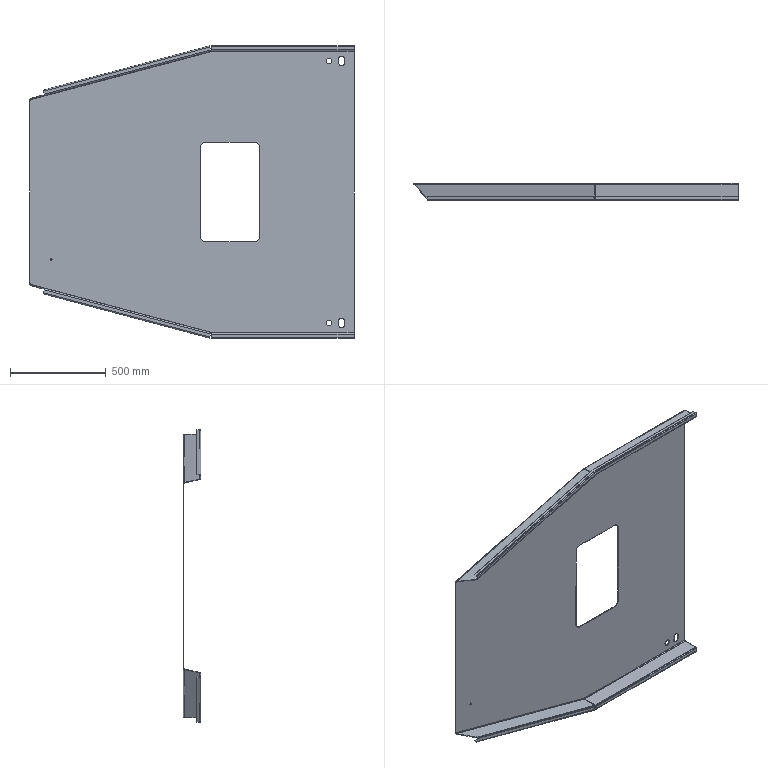Part | SolidWorks | features EdgeFlange 3, ICE 2, FlatPattern 1, MirrorPattern 1, SMBaseFlange 1, SheetMetal 1 | 1 solid | 141 faces | box 1688 x 90 x 1525 mm | volume 7493829 mm3 | plane 90 | cylinder 45 | spline 6 | commonest cylinder face diameters 6 x12 12 x12 30 x10 1.5 x5 56 x4 10 x2